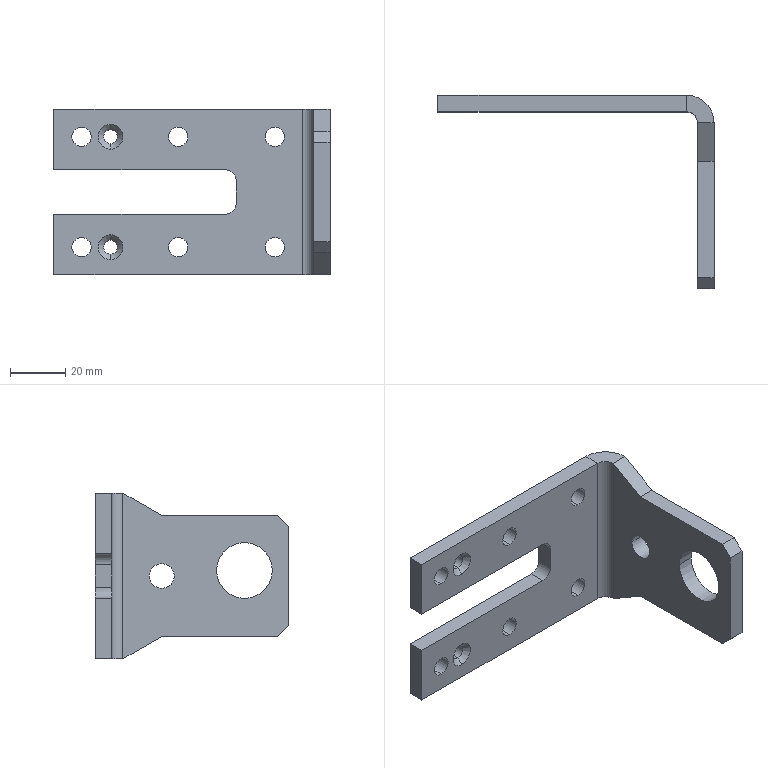Part | STEP file | Ngam kep 7 | 1 solid | 48 faces | box 100 x 70 x 60 mm | volume 42428 mm3 | cylinder 24 | plane 20 | cone 4 | commonest cylinder face diameters 7 x12 5 x4 8 x3 9 x2 20.2 x2 20 x1